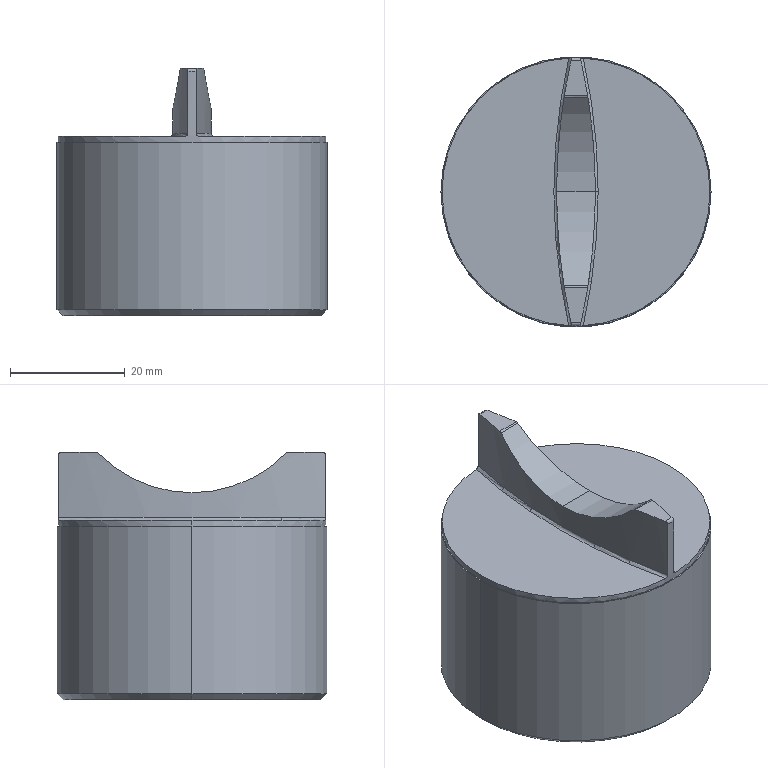Part | SolidWorks | features Fillet 3, ICE 3, Chamfer 1, Extrusion 1, HoleWzd 1 | 1 solid | 28 faces | box 47 x 47 x 43 mm | volume 54544 mm3 | cylinder 13 | plane 6 | torus 5 | cone 4 | commonest cylinder face diameters 210.861 x3 1 x2 8.5 x2 45.893 x2 46.6 x2 47 x2
STEP:
#1=CARTESIAN_POINT('',(-22.5,0.,0.));
#2=VERTEX_POINT('',#1);
#3=CARTESIAN_POINT('',(22.5,0.,0.));
#4=VERTEX_POINT('',#3);
#5=CARTESIAN_POINT('',(0.,0.,0.));
#6=DIRECTION('',(0.,0.,-1.));
#7=DIRECTION('',(1.,0.,0.));
#8=AXIS2_PLACEMENT_3D('',#5,#6,#7);
#9=CIRCLE('',#8,22.5);
#10=EDGE_CURVE('',#2,#4,#9,.T.);
#11=ORIENTED_EDGE('',*,*,#10,.F.);
#12=CARTESIAN_POINT('',(-23.5,0.,1.));
#13=VERTEX_POINT('',#12);
#14=CARTESIAN_POINT('',(-23.5,0.,1.));
#15=DIRECTION('',(-0.7071,0.,0.7071));
#16=VECTOR('',#15,1000.);
#17=LINE('',#14,#16);
#18=EDGE_CURVE('',#2,#13,#17,.T.);
#19=ORIENTED_EDGE('',*,*,#18,.T.);
#20=CARTESIAN_POINT('',(23.5,0.,1.));
#21=VERTEX_POINT('',#20);
#22=CARTESIAN_POINT('',(0.,0.,1.));
#23=DIRECTION('',(0.,0.,1.));
#24=DIRECTION('',(1.,0.,0.));
#25=AXIS2_PLACEMENT_3D('',#22,#23,#24);
#26=CIRCLE('',#25,23.5);
#27=EDGE_CURVE('',#21,#13,#26,.T.);
#28=ORIENTED_EDGE('',*,*,#27,.F.);
#29=CARTESIAN_POINT('',(23.5,0.,1.));
#30=DIRECTION('',(0.7071,0.,0.7071));
#31=VECTOR('',#30,1000.);
#32=LINE('',#29,#31);
#33=EDGE_CURVE('',#4,#21,#32,.T.);
#34=ORIENTED_EDGE('',*,*,#33,.F.);
#35=EDGE_LOOP('',(#11,#19,#28,#34));
#36=FACE_OUTER_BOUND('',#35,.T.);
#37=CARTESIAN_POINT('',(0.,0.,1.));
#38=DIRECTION('',(0.,0.,1.));
#39=DIRECTION('',(1.,0.,0.));
#40=AXIS2_PLACEMENT_3D('',#37,#38,#39);
#41=CONICAL_SURFACE('',#40,23.5,0.7854);
#42=ADVANCED_FACE('',(#36),#41,.T.);
#43=CARTESIAN_POINT('',(0.7458,-23.288,31.7));
#44=VERTEX_POINT('',#43);
#45=CARTESIAN_POINT('',(3.35,0.,31.7));
#46=VERTEX_POINT('',#45);
#47=CARTESIAN_POINT('',(-102.081,0.,31.7));
#48=DIRECTION('',(0.,0.,1.));
#49=DIRECTION('',(1.,0.,0.));
#50=AXIS2_PLACEMENT_3D('',#47,#48,#49);
#51=CIRCLE('',#50,105.431);
#52=EDGE_CURVE('',#44,#46,#51,.T.);
#53=ORIENTED_EDGE('',*,*,#52,.T.);
#54=CARTESIAN_POINT('',(3.35,0.,36.));
#55=VERTEX_POINT('',#54);
#56=CARTESIAN_POINT('',(3.35,0.,31.2));
#57=DIRECTION('',(0.,0.,1.));
#58=VECTOR('',#57,1000.);
#59=LINE('',#56,#58);
#60=EDGE_CURVE('',#46,#55,#59,.T.);
#61=ORIENTED_EDGE('',*,*,#60,.T.);
#62=CARTESIAN_POINT('',(2.074,-16.354,42.851));
#63=VERTEX_POINT('',#62);
#64=CARTESIAN_POINT('',(2.074,-16.354,42.851));
#65=CARTESIAN_POINT('',(2.242,-15.285,41.764));
#66=CARTESIAN_POINT('',(2.407,-14.125,40.8));
#67=CARTESIAN_POINT('',(2.637,-12.253,39.531));
#68=CARTESIAN_POINT('',(2.711,-11.607,39.137));
#69=CARTESIAN_POINT('',(2.816,-10.603,38.593));
#70=CARTESIAN_POINT('',(2.85,-10.262,38.419));
#71=CARTESIAN_POINT('',(2.915,-9.574,38.089));
#72=CARTESIAN_POINT('',(2.946,-9.227,37.933));
#73=CARTESIAN_POINT('',(3.094,-7.478,37.2));
#74=CARTESIAN_POINT('',(3.188,-6.034,36.755));
#75=CARTESIAN_POINT('',(3.268,-4.172,36.379));
#76=CARTESIAN_POINT('',(3.282,-3.797,36.313));
#77=CARTESIAN_POINT('',(3.307,-3.04,36.199));
#78=CARTESIAN_POINT('',(3.317,-2.658,36.151));
#79=CARTESIAN_POINT('',(3.342,-1.517,36.037));
#80=CARTESIAN_POINT('',(3.35,-0.7577,36.));
#81=CARTESIAN_POINT('',(3.35,0.,36.));
#82=B_SPLINE_CURVE_WITH_KNOTS('',3,(#64,#65,#66,#67,#68,#69,#70,#71,#72,#73,#74,#75,#76,#77,#78,#79,#80,#81),.UNSPECIFIED.,.F.,.F.,(4,2,2,2,2,2,2,2,4),(0.000207,0.004751,0.007022,0.008158,0.009294,0.01384,0.01497,0.01611,0.01838),.UNSPECIFIED.);
#83=EDGE_CURVE('',#63,#55,#82,.T.);
#84=ORIENTED_EDGE('',*,*,#83,.F.);
#85=CARTESIAN_POINT('',(2.017,-16.711,43.));
#86=VERTEX_POINT('',#85);
#87=CARTESIAN_POINT('',(2.074,-16.354,42.851));
#88=CARTESIAN_POINT('',(2.059,-16.448,42.946));
#89=CARTESIAN_POINT('',(2.039,-16.578,43.));
#90=CARTESIAN_POINT('',(2.017,-16.711,43.));
#91=B_SPLINE_CURVE_WITH_KNOTS('',3,(#87,#88,#89,#90),.UNSPECIFIED.,.F.,.F.,(4,4),(0.,0.0003983),.UNSPECIFIED.);
#92=EDGE_CURVE('',#63,#86,#91,.T.);
#93=ORIENTED_EDGE('',*,*,#92,.T.);
#94=CARTESIAN_POINT('',(0.8587,-22.784,43.));
#95=VERTEX_POINT('',#94);
#96=CARTESIAN_POINT('',(-102.081,0.,43.));
#97=DIRECTION('',(0.,0.,1.));
#98=DIRECTION('',(1.,0.,0.));
#99=AXIS2_PLACEMENT_3D('',#96,#97,#98);
#100=CIRCLE('',#99,105.431);
#101=EDGE_CURVE('',#95,#86,#100,.T.);
#102=ORIENTED_EDGE('',*,*,#101,.F.);
#103=CARTESIAN_POINT('',(0.7458,-23.288,42.5));
#104=VERTEX_POINT('',#103);
#105=CARTESIAN_POINT('',(0.8587,-22.784,43.));
#106=CARTESIAN_POINT('',(0.8297,-22.915,43.));
#107=CARTESIAN_POINT('',(0.801,-23.043,42.948));
#108=CARTESIAN_POINT('',(0.7587,-23.231,42.765));
#109=CARTESIAN_POINT('',(0.7458,-23.288,42.634));
#110=CARTESIAN_POINT('',(0.7458,-23.288,42.5));
#111=B_SPLINE_CURVE_WITH_KNOTS('',3,(#105,#106,#107,#108,#109,#110),.UNSPECIFIED.,.F.,.F.,(4,2,4),(0.,0.0003971,0.0007942),.UNSPECIFIED.);
#112=EDGE_CURVE('',#95,#104,#111,.T.);
#113=ORIENTED_EDGE('',*,*,#112,.T.);
#114=CARTESIAN_POINT('',(0.7458,-23.288,96.2));
#115=DIRECTION('',(0.,0.,1.));
#116=VECTOR('',#115,1000.);
#117=LINE('',#114,#116);
#118=EDGE_CURVE('',#44,#104,#117,.T.);
#119=ORIENTED_EDGE('',*,*,#118,.F.);
#120=EDGE_LOOP('',(#53,#61,#84,#93,#102,#113,#119));
#121=FACE_OUTER_BOUND('',#120,.T.);
#122=CARTESIAN_POINT('',(-102.081,0.,31.2));
#123=DIRECTION('',(0.,0.,1.));
#124=DIRECTION('',(1.,0.,0.));
#125=AXIS2_PLACEMENT_3D('',#122,#123,#124);
#126=CYLINDRICAL_SURFACE('',#125,105.431);
#127=ADVANCED_FACE('',(#121),#126,.T.);
#128=CARTESIAN_POINT('',(-3.35,0.,36.));
#129=VERTEX_POINT('',#128);
#130=CARTESIAN_POINT('',(-2.074,16.354,42.851));
#131=VERTEX_POINT('',#130);
#132=CARTESIAN_POINT('',(-3.35,0.,36.));
#133=CARTESIAN_POINT('',(-3.35,1.514,36.));
#134=CARTESIAN_POINT('',(-3.317,3.022,36.148));
#135=CARTESIAN_POINT('',(-3.221,5.274,36.601));
#136=CARTESIAN_POINT('',(-3.181,6.014,36.789));
#137=CARTESIAN_POINT('',(-3.088,7.462,37.234));
#138=CARTESIAN_POINT('',(-3.035,8.172,37.491));
#139=CARTESIAN_POINT('',(-2.918,9.565,38.075));
#140=CARTESIAN_POINT('',(-2.853,10.247,38.401));
#141=CARTESIAN_POINT('',(-2.714,11.584,39.124));
#142=CARTESIAN_POINT('',(-2.639,12.239,39.521));
#143=CARTESIAN_POINT('',(-2.407,14.123,40.798));
#144=CARTESIAN_POINT('',(-2.242,15.286,41.765));
#145=CARTESIAN_POINT('',(-2.074,16.354,42.851));
#146=B_SPLINE_CURVE_WITH_KNOTS('',3,(#132,#133,#134,#135,#136,#137,#138,#139,#140,#141,#142,#143,#144,#145),.UNSPECIFIED.,.F.,.F.,(4,2,2,2,2,2,4),(0.01838,0.02292,0.02519,0.02746,0.02973,0.032,0.03654),.UNSPECIFIED.);
#147=EDGE_CURVE('',#129,#131,#146,.T.);
#148=ORIENTED_EDGE('',*,*,#147,.F.);
#149=CARTESIAN_POINT('',(-6.,0.,36.));
#150=DIRECTION('',(1.,0.,0.));
#151=VECTOR('',#150,1000.);
#152=LINE('',#149,#151);
#153=EDGE_CURVE('',#129,#55,#152,.T.);
#154=ORIENTED_EDGE('',*,*,#153,.T.);
#155=CARTESIAN_POINT('',(2.074,16.354,42.851));
#156=VERTEX_POINT('',#155);
#157=CARTESIAN_POINT('',(3.35,0.,36.));
#158=CARTESIAN_POINT('',(3.35,1.514,36.));
#159=CARTESIAN_POINT('',(3.317,3.022,36.148));
#160=CARTESIAN_POINT('',(3.221,5.274,36.601));
#161=CARTESIAN_POINT('',(3.181,6.014,36.789));
#162=CARTESIAN_POINT('',(3.088,7.462,37.234));
#163=CARTESIAN_POINT('',(3.035,8.172,37.491));
#164=CARTESIAN_POINT('',(2.918,9.565,38.075));
#165=CARTESIAN_POINT('',(2.853,10.247,38.401));
#166=CARTESIAN_POINT('',(2.714,11.584,39.124));
#167=CARTESIAN_POINT('',(2.639,12.239,39.521));
#168=CARTESIAN_POINT('',(2.407,14.123,40.798));
#169=CARTESIAN_POINT('',(2.242,15.286,41.765));
#170=CARTESIAN_POINT('',(2.074,16.354,42.851));
#171=B_SPLINE_CURVE_WITH_KNOTS('',3,(#157,#158,#159,#160,#161,#162,#163,#164,#165,#166,#167,#168,#169,#170),.UNSPECIFIED.,.F.,.F.,(4,2,2,2,2,2,4),(0.01838,0.02292,0.02519,0.02746,0.02973,0.032,0.03654),.UNSPECIFIED.);
#172=EDGE_CURVE('',#55,#156,#171,.T.);
#173=ORIENTED_EDGE('',*,*,#172,.T.);
#174=CARTESIAN_POINT('',(-6.,16.354,42.851));
#175=DIRECTION('',(-1.,0.,0.));
#176=VECTOR('',#175,1000.);
#177=LINE('',#174,#176);
#178=EDGE_CURVE('',#156,#131,#177,.T.);
#179=ORIENTED_EDGE('',*,*,#178,.T.);
#180=EDGE_LOOP('',(#148,#154,#173,#179));
#181=FACE_OUTER_BOUND('',#180,.T.);
#182=CARTESIAN_POINT('',(-6.,0.,58.946));
#183=DIRECTION('',(1.,0.,0.));
#184=DIRECTION('',(0.,0.,-1.));
#185=AXIS2_PLACEMENT_3D('',#182,#183,#184);
#186=CYLINDRICAL_SURFACE('',#185,22.946);
#187=ADVANCED_FACE('',(#181),#186,.F.);
#188=CARTESIAN_POINT('',(1.263,23.266,31.2));
#189=VERTEX_POINT('',#188);
#190=CARTESIAN_POINT('',(23.3,0.,31.2));
#191=VERTEX_POINT('',#190);
#192=CARTESIAN_POINT('',(0.,0.,31.2));
#193=DIRECTION('',(0.,0.,-1.));
#194=DIRECTION('',(1.,0.,0.));
#195=AXIS2_PLACEMENT_3D('',#192,#193,#194);
#196=CIRCLE('',#195,23.3);
#197=EDGE_CURVE('',#189,#191,#196,.T.);
#198=ORIENTED_EDGE('',*,*,#197,.T.);
#199=CARTESIAN_POINT('',(23.3,0.,30.2));
#200=VERTEX_POINT('',#199);
#201=CARTESIAN_POINT('',(23.3,0.,162.2));
#202=DIRECTION('',(0.,0.,-1.));
#203=VECTOR('',#202,1000.);
#204=LINE('',#201,#203);
#205=EDGE_CURVE('',#191,#200,#204,.T.);
#206=ORIENTED_EDGE('',*,*,#205,.T.);
#207=CARTESIAN_POINT('',(-23.3,0.,30.2));
#208=VERTEX_POINT('',#207);
#209=CARTESIAN_POINT('',(0.,0.,30.2));
#210=DIRECTION('',(0.,0.,1.));
#211=DIRECTION('',(1.,0.,0.));
#212=AXIS2_PLACEMENT_3D('',#209,#210,#211);
#213=CIRCLE('',#212,23.3);
#214=EDGE_CURVE('',#200,#208,#213,.T.);
#215=ORIENTED_EDGE('',*,*,#214,.T.);
#216=CARTESIAN_POINT('',(-23.3,0.,31.2));
#217=VERTEX_POINT('',#216);
#218=CARTESIAN_POINT('',(-23.3,0.,162.2));
#219=DIRECTION('',(0.,0.,-1.));
#220=VECTOR('',#219,1000.);
#221=LINE('',#218,#220);
#222=EDGE_CURVE('',#217,#208,#221,.T.);
#223=ORIENTED_EDGE('',*,*,#222,.F.);
#224=CARTESIAN_POINT('',(-1.263,23.266,31.2));
#225=VERTEX_POINT('',#224);
#226=CARTESIAN_POINT('',(0.,0.,31.2));
#227=DIRECTION('',(0.,0.,-1.));
#228=DIRECTION('',(1.,0.,0.));
#229=AXIS2_PLACEMENT_3D('',#226,#227,#228);
#230=CIRCLE('',#229,23.3);
#231=EDGE_CURVE('',#217,#225,#230,.T.);
#232=ORIENTED_EDGE('',*,*,#231,.T.);
#233=CARTESIAN_POINT('',(-0.7458,23.288,31.7));
#234=VERTEX_POINT('',#233);
#235=CARTESIAN_POINT('',(-0.7458,23.288,31.7));
#236=CARTESIAN_POINT('',(-0.7458,23.288,31.567));
#237=CARTESIAN_POINT('',(-0.804,23.286,31.435));
#238=CARTESIAN_POINT('',(-0.9971,23.279,31.252));
#239=CARTESIAN_POINT('',(-1.129,23.273,31.2));
#240=CARTESIAN_POINT('',(-1.263,23.266,31.2));
#241=B_SPLINE_CURVE_WITH_KNOTS('',3,(#235,#236,#237,#238,#239,#240),.UNSPECIFIED.,.F.,.F.,(4,2,4),(0.00007147,0.0004697,0.000868),.UNSPECIFIED.);
#242=EDGE_CURVE('',#234,#225,#241,.T.);
#243=ORIENTED_EDGE('',*,*,#242,.F.);
#244=CARTESIAN_POINT('',(-0.7458,23.288,42.5));
#245=VERTEX_POINT('',#244);
#246=CARTESIAN_POINT('',(-0.7458,23.288,96.2));
#247=DIRECTION('',(0.,0.,-1.));
#248=VECTOR('',#247,1000.);
#249=LINE('',#246,#248);
#250=EDGE_CURVE('',#245,#234,#249,.T.);
#251=ORIENTED_EDGE('',*,*,#250,.F.);
#252=CARTESIAN_POINT('',(0.7458,23.288,42.5));
#253=VERTEX_POINT('',#252);
#254=CARTESIAN_POINT('',(0.,0.,42.5));
#255=DIRECTION('',(0.,0.,-1.));
#256=DIRECTION('',(1.,0.,0.));
#257=AXIS2_PLACEMENT_3D('',#254,#255,#256);
#258=CIRCLE('',#257,23.3);
#259=EDGE_CURVE('',#245,#253,#258,.T.);
#260=ORIENTED_EDGE('',*,*,#259,.T.);
#261=CARTESIAN_POINT('',(0.7458,23.288,31.7));
#262=VERTEX_POINT('',#261);
#263=CARTESIAN_POINT('',(0.7458,23.288,96.2));
#264=DIRECTION('',(0.,0.,-1.));
#265=VECTOR('',#264,1000.);
#266=LINE('',#263,#265);
#267=EDGE_CURVE('',#253,#262,#266,.T.);
#268=ORIENTED_EDGE('',*,*,#267,.T.);
#269=CARTESIAN_POINT('',(1.263,23.266,31.2));
#270=CARTESIAN_POINT('',(1.131,23.273,31.2));
#271=CARTESIAN_POINT('',(0.9971,23.279,31.252));
#272=CARTESIAN_POINT('',(0.8044,23.286,31.434));
#273=CARTESIAN_POINT('',(0.7458,23.288,31.565));
#274=CARTESIAN_POINT('',(0.7458,23.288,31.7));
#275=B_SPLINE_CURVE_WITH_KNOTS('',3,(#269,#270,#271,#272,#273,#274),.UNSPECIFIED.,.F.,.F.,(4,2,4),(0.00004476,0.0004428,0.0008408),.UNSPECIFIED.);
#276=EDGE_CURVE('',#189,#262,#275,.T.);
#277=ORIENTED_EDGE('',*,*,#276,.F.);
#278=EDGE_LOOP('',(#198,#206,#215,#223,#232,#243,#251,#260,#268,#277));
#279=FACE_OUTER_BOUND('',#278,.T.);
#280=CARTESIAN_POINT('',(0.,0.,162.2));
#281=DIRECTION('',(0.,0.,-1.));
#282=DIRECTION('',(-1.,0.,0.));
#283=AXIS2_PLACEMENT_3D('',#280,#281,#282);
#284=CYLINDRICAL_SURFACE('',#283,23.3);
#285=ADVANCED_FACE('',(#279),#284,.T.);
#286=CARTESIAN_POINT('',(4.25,0.,21.));
#287=VERTEX_POINT('',#286);
#288=CARTESIAN_POINT('',(-4.25,0.,21.));
#289=VERTEX_POINT('',#288);
#290=CARTESIAN_POINT('',(0.,0.,21.));
#291=DIRECTION('',(0.,0.,-1.));
#292=DIRECTION('',(-1.,0.,0.));
#293=AXIS2_PLACEMENT_3D('',#290,#291,#292);
#294=CIRCLE('',#293,4.25);
#295=EDGE_CURVE('',#287,#289,#294,.T.);
#296=ORIENTED_EDGE('',*,*,#295,.F.);
#297=CARTESIAN_POINT('',(4.25,0.,0.));
#298=VERTEX_POINT('',#297);
#299=CARTESIAN_POINT('',(4.25,0.,0.));
#300=DIRECTION('',(0.,0.,-1.));
#301=VECTOR('',#300,1000.);
#302=LINE('',#299,#301);
#303=EDGE_CURVE('',#287,#298,#302,.T.);
#304=ORIENTED_EDGE('',*,*,#303,.T.);
#305=CARTESIAN_POINT('',(-4.25,0.,0.));
#306=VERTEX_POINT('',#305);
#307=CARTESIAN_POINT('',(0.,0.,0.));
#308=DIRECTION('',(0.,0.,-1.));
#309=DIRECTION('',(-1.,0.,0.));
#310=AXIS2_PLACEMENT_3D('',#307,#308,#309);
#311=CIRCLE('',#310,4.25);
#312=EDGE_CURVE('',#298,#306,#311,.T.);
#313=ORIENTED_EDGE('',*,*,#312,.T.);
#314=CARTESIAN_POINT('',(-4.25,0.,0.));
#315=DIRECTION('',(0.,0.,-1.));
#316=VECTOR('',#315,1000.);
#317=LINE('',#314,#316);
#318=EDGE_CURVE('',#289,#306,#317,.T.);
#319=ORIENTED_EDGE('',*,*,#318,.F.);
#320=EDGE_LOOP('',(#296,#304,#313,#319));
#321=FACE_OUTER_BOUND('',#320,.T.);
#322=CARTESIAN_POINT('',(0.,0.,0.));
#323=DIRECTION('',(0.,0.,-1.));
#324=DIRECTION('',(-1.,0.,0.));
#325=AXIS2_PLACEMENT_3D('',#322,#323,#324);
#326=CYLINDRICAL_SURFACE('',#325,4.25);
#327=ADVANCED_FACE('',(#321),#326,.F.);
#328=CARTESIAN_POINT('',(0.,0.,23.554));
#329=VERTEX_POINT('',#328);
#330=CARTESIAN_POINT('',(-4.25,0.,21.));
#331=DIRECTION('',(-0.8572,0.,-0.515));
#332=VECTOR('',#331,1000.);
#333=LINE('',#330,#332);
#334=EDGE_CURVE('',#329,#289,#333,.T.);
#335=ORIENTED_EDGE('',*,*,#334,.F.);
#336=CARTESIAN_POINT('',(4.25,0.,21.));
#337=DIRECTION('',(0.8572,0.,-0.515));
#338=VECTOR('',#337,1000.);
#339=LINE('',#336,#338);
#340=EDGE_CURVE('',#329,#287,#339,.T.);
#341=ORIENTED_EDGE('',*,*,#340,.T.);
#342=ORIENTED_EDGE('',*,*,#295,.T.);
#343=EDGE_LOOP('',(#335,#341,#342));
#344=FACE_OUTER_BOUND('',#343,.T.);
#345=CARTESIAN_POINT('',(0.,0.,21.));
#346=DIRECTION('',(0.,0.,-1.));
#347=DIRECTION('',(-1.,0.,0.));
#348=AXIS2_PLACEMENT_3D('',#345,#346,#347);
#349=CONICAL_SURFACE('',#348,4.25,1.03);
#350=ADVANCED_FACE('',(#344),#349,.F.);
#351=CARTESIAN_POINT('',(23.5,0.,30.2));
#352=VERTEX_POINT('',#351);
#353=CARTESIAN_POINT('',(-23.5,0.,30.2));
#354=VERTEX_POINT('',#353);
#355=CARTESIAN_POINT('',(0.,0.,30.2));
#356=DIRECTION('',(0.,0.,1.));
#357=DIRECTION('',(1.,0.,0.));
#358=AXIS2_PLACEMENT_3D('',#355,#356,#357);
#359=CIRCLE('',#358,23.5);
#360=EDGE_CURVE('',#352,#354,#359,.T.);
#361=ORIENTED_EDGE('',*,*,#360,.F.);
#362=CARTESIAN_POINT('',(23.5,0.,43.));
#363=DIRECTION('',(0.,0.,-1.));
#364=VECTOR('',#363,1000.);
#365=LINE('',#362,#364);
#366=EDGE_CURVE('',#352,#21,#365,.T.);
#367=ORIENTED_EDGE('',*,*,#366,.T.);
#368=ORIENTED_EDGE('',*,*,#27,.T.);
#369=CARTESIAN_POINT('',(-23.5,0.,43.));
#370=DIRECTION('',(0.,0.,-1.));
#371=VECTOR('',#370,1000.);
#372=LINE('',#369,#371);
#373=EDGE_CURVE('',#354,#13,#372,.T.);
#374=ORIENTED_EDGE('',*,*,#373,.F.);
#375=EDGE_LOOP('',(#361,#367,#368,#374));
#376=FACE_OUTER_BOUND('',#375,.T.);
#377=CARTESIAN_POINT('',(0.,0.,43.));
#378=DIRECTION('',(0.,0.,-1.));
#379=DIRECTION('',(-1.,0.,0.));
#380=AXIS2_PLACEMENT_3D('',#377,#378,#379);
#381=CYLINDRICAL_SURFACE('',#380,23.5);
#382=ADVANCED_FACE('',(#376),#381,.T.);
#383=CARTESIAN_POINT('',(-102.081,0.,31.7));
#384=DIRECTION('',(0.,0.,1.));
#385=DIRECTION('',(1.,0.,0.));
#386=AXIS2_PLACEMENT_3D('',#383,#384,#385);
#387=CIRCLE('',#386,105.431);
#388=EDGE_CURVE('',#46,#262,#387,.T.);
#389=ORIENTED_EDGE('',*,*,#388,.F.);
#390=CARTESIAN_POINT('',(3.85,0.,31.2));
#391=VERTEX_POINT('',#390);
#392=CARTESIAN_POINT('',(3.85,0.,31.7));
#393=DIRECTION('',(0.,-1.,0.));
#394=DIRECTION('',(0.,0.,-1.));
#395=AXIS2_PLACEMENT_3D('',#392,#393,#394);
#396=CIRCLE('',#395,0.5);
#397=EDGE_CURVE('',#46,#391,#396,.T.);
#398=ORIENTED_EDGE('',*,*,#397,.T.);
#399=CARTESIAN_POINT('',(-102.081,0.,31.2));
#400=DIRECTION('',(0.,0.,-1.));
#401=DIRECTION('',(1.,0.,0.));
#402=AXIS2_PLACEMENT_3D('',#399,#400,#401);
#403=CIRCLE('',#402,105.931);
#404=EDGE_CURVE('',#189,#391,#403,.T.);
#405=ORIENTED_EDGE('',*,*,#404,.F.);
#406=ORIENTED_EDGE('',*,*,#276,.T.);
#407=EDGE_LOOP('',(#389,#398,#405,#406));
#408=FACE_OUTER_BOUND('',#407,.T.);
#409=CARTESIAN_POINT('',(-102.081,0.,31.7));
#410=DIRECTION('',(0.,0.,1.));
#411=DIRECTION('',(1.,0.,0.));
#412=AXIS2_PLACEMENT_3D('',#409,#410,#411);
#413=TOROIDAL_SURFACE('',#412,105.931,0.5);
#414=ADVANCED_FACE('',(#408),#413,.F.);
#415=CARTESIAN_POINT('',(-0.7458,-23.288,31.7));
#416=VERTEX_POINT('',#415);
#417=CARTESIAN_POINT('',(102.081,0.,31.7));
#418=DIRECTION('',(0.,0.,1.));
#419=DIRECTION('',(1.,0.,0.));
#420=AXIS2_PLACEMENT_3D('',#417,#418,#419);
#421=CIRCLE('',#420,105.431);
#422=EDGE_CURVE('',#234,#416,#421,.T.);
#423=ORIENTED_EDGE('',*,*,#422,.F.);
#424=ORIENTED_EDGE('',*,*,#242,.T.);
#425=CARTESIAN_POINT('',(-1.263,-23.266,31.2));
#426=VERTEX_POINT('',#425);
#427=CARTESIAN_POINT('',(102.081,0.,31.2));
#428=DIRECTION('',(0.,0.,-1.));
#429=DIRECTION('',(1.,0.,0.));
#430=AXIS2_PLACEMENT_3D('',#427,#428,#429);
#431=CIRCLE('',#430,105.931);
#432=EDGE_CURVE('',#426,#225,#431,.T.);
#433=ORIENTED_EDGE('',*,*,#432,.F.);
#434=CARTESIAN_POINT('',(-1.263,-23.266,31.2));
#435=CARTESIAN_POINT('',(-1.131,-23.273,31.2));
#436=CARTESIAN_POINT('',(-0.9971,-23.279,31.252));
#437=CARTESIAN_POINT('',(-0.8044,-23.286,31.434));
#438=CARTESIAN_POINT('',(-0.7458,-23.288,31.565));
#439=CARTESIAN_POINT('',(-0.7458,-23.288,31.7));
#440=B_SPLINE_CURVE_WITH_KNOTS('',3,(#434,#435,#436,#437,#438,#439),.UNSPECIFIED.,.F.,.F.,(4,2,4),(0.00004476,0.0004428,0.0008408),.UNSPECIFIED.);
#441=EDGE_CURVE('',#426,#416,#440,.T.);
#442=ORIENTED_EDGE('',*,*,#441,.T.);
#443=EDGE_LOOP('',(#423,#424,#433,#442));
#444=FACE_OUTER_BOUND('',#443,.T.);
#445=CARTESIAN_POINT('',(102.081,0.,31.7));
#446=DIRECTION('',(0.,0.,1.));
#447=DIRECTION('',(1.,0.,0.));
#448=AXIS2_PLACEMENT_3D('',#445,#446,#447);
#449=TOROIDAL_SURFACE('',#448,105.931,0.5);
#450=ADVANCED_FACE('',(#444),#449,.F.);
#451=ORIENTED_EDGE('',*,*,#397,.F.);
#452=ORIENTED_EDGE('',*,*,#52,.F.);
#453=CARTESIAN_POINT('',(1.263,-23.266,31.2));
#454=VERTEX_POINT('',#453);
#455=CARTESIAN_POINT('',(0.7458,-23.288,31.7));
#456=CARTESIAN_POINT('',(0.7458,-23.288,31.567));
#457=CARTESIAN_POINT('',(0.804,-23.286,31.435));
#458=CARTESIAN_POINT('',(0.9971,-23.279,31.252));
#459=CARTESIAN_POINT('',(1.129,-23.273,31.2));
#460=CARTESIAN_POINT('',(1.263,-23.266,31.2));
#461=B_SPLINE_CURVE_WITH_KNOTS('',3,(#455,#456,#457,#458,#459,#460),.UNSPECIFIED.,.F.,.F.,(4,2,4),(0.00007147,0.0004697,0.000868),.UNSPECIFIED.);
#462=EDGE_CURVE('',#44,#454,#461,.T.);
#463=ORIENTED_EDGE('',*,*,#462,.T.);
#464=CARTESIAN_POINT('',(-102.081,0.,31.2));
#465=DIRECTION('',(0.,0.,-1.));
#466=DIRECTION('',(1.,0.,0.));
#467=AXIS2_PLACEMENT_3D('',#464,#465,#466);
#468=CIRCLE('',#467,105.931);
#469=EDGE_CURVE('',#391,#454,#468,.T.);
#470=ORIENTED_EDGE('',*,*,#469,.F.);
#471=EDGE_LOOP('',(#451,#452,#463,#470));
#472=FACE_OUTER_BOUND('',#471,.T.);
#473=CARTESIAN_POINT('',(-102.081,0.,31.7));
#474=DIRECTION('',(0.,0.,1.));
#475=DIRECTION('',(1.,0.,0.));
#476=AXIS2_PLACEMENT_3D('',#473,#474,#475);
#477=TOROIDAL_SURFACE('',#476,105.931,0.5);
#478=ADVANCED_FACE('',(#472),#477,.F.);
#479=ORIENTED_EDGE('',*,*,#366,.F.);
#480=CARTESIAN_POINT('',(0.,0.,30.2));
#481=DIRECTION('',(0.,0.,1.));
#482=DIRECTION('',(1.,0.,0.));
#483=AXIS2_PLACEMENT_3D('',#480,#481,#482);
#484=CIRCLE('',#483,23.5);
#485=EDGE_CURVE('',#354,#352,#484,.T.);
#486=ORIENTED_EDGE('',*,*,#485,.F.);
#487=ORIENTED_EDGE('',*,*,#373,.T.);
#488=CARTESIAN_POINT('',(0.,0.,1.));
#489=DIRECTION('',(0.,0.,1.));
#490=DIRECTION('',(1.,0.,0.));
#491=AXIS2_PLACEMENT_3D('',#488,#489,#490);
#492=CIRCLE('',#491,23.5);
#493=EDGE_CURVE('',#13,#21,#492,.T.);
#494=ORIENTED_EDGE('',*,*,#493,.T.);
#495=EDGE_LOOP('',(#479,#486,#487,#494));
#496=FACE_OUTER_BOUND('',#495,.T.);
#497=CARTESIAN_POINT('',(0.,0.,43.));
#498=DIRECTION('',(0.,0.,-1.));
#499=DIRECTION('',(-1.,0.,0.));
#500=AXIS2_PLACEMENT_3D('',#497,#498,#499);
#501=CYLINDRICAL_SURFACE('',#500,23.5);
#502=ADVANCED_FACE('',(#496),#501,.T.);
#503=CARTESIAN_POINT('',(0.,0.,0.));
#504=DIRECTION('',(0.,0.,-1.));
#505=DIRECTION('',(1.,0.,0.));
#506=AXIS2_PLACEMENT_3D('',#503,#504,#505);
#507=CIRCLE('',#506,22.5);
#508=EDGE_CURVE('',#4,#2,#507,.T.);
#509=ORIENTED_EDGE('',*,*,#508,.T.);
#510=ORIENTED_EDGE('',*,*,#10,.T.);
#511=EDGE_LOOP('',(#509,#510));
#512=FACE_OUTER_BOUND('',#511,.T.);
#513=CARTESIAN_POINT('',(0.,0.,0.));
#514=DIRECTION('',(0.,0.,-1.));
#515=DIRECTION('',(-1.,0.,0.));
#516=AXIS2_PLACEMENT_3D('',#513,#514,#515);
#517=CIRCLE('',#516,4.25);
#518=EDGE_CURVE('',#306,#298,#517,.T.);
#519=ORIENTED_EDGE('',*,*,#518,.F.);
#520=ORIENTED_EDGE('',*,*,#312,.F.);
#521=EDGE_LOOP('',(#519,#520));
#522=FACE_BOUND('',#521,.T.);
#523=CARTESIAN_POINT('',(0.,0.,0.));
#524=DIRECTION('',(0.,0.,1.));
#525=DIRECTION('',(1.,0.,0.));
#526=AXIS2_PLACEMENT_3D('',#523,#524,#525);
#527=PLANE('',#526);
#528=ADVANCED_FACE('',(#512,#522),#527,.F.);
#529=ORIENTED_EDGE('',*,*,#340,.F.);
#530=ORIENTED_EDGE('',*,*,#334,.T.);
#531=CARTESIAN_POINT('',(0.,0.,21.));
#532=DIRECTION('',(0.,0.,-1.));
#533=DIRECTION('',(-1.,0.,0.));
#534=AXIS2_PLACEMENT_3D('',#531,#532,#533);
#535=CIRCLE('',#534,4.25);
#536=EDGE_CURVE('',#289,#287,#535,.T.);
#537=ORIENTED_EDGE('',*,*,#536,.T.);
#538=EDGE_LOOP('',(#529,#530,#537));
#539=FACE_OUTER_BOUND('',#538,.T.);
#540=CARTESIAN_POINT('',(0.,0.,21.));
#541=DIRECTION('',(0.,0.,-1.));
#542=DIRECTION('',(-1.,0.,0.));
#543=AXIS2_PLACEMENT_3D('',#540,#541,#542);
#544=CONICAL_SURFACE('',#543,4.25,1.03);
#545=ADVANCED_FACE('',(#539),#544,.F.);
#546=ORIENTED_EDGE('',*,*,#303,.F.);
#547=ORIENTED_EDGE('',*,*,#536,.F.);
#548=ORIENTED_EDGE('',*,*,#318,.T.);
#549=ORIENTED_EDGE('',*,*,#518,.T.);
#550=EDGE_LOOP('',(#546,#547,#548,#549));
#551=FACE_OUTER_BOUND('',#550,.T.);
#552=CARTESIAN_POINT('',(0.,0.,0.));
#553=DIRECTION('',(0.,0.,-1.));
#554=DIRECTION('',(-1.,0.,0.));
#555=AXIS2_PLACEMENT_3D('',#552,#553,#554);
#556=CYLINDRICAL_SURFACE('',#555,4.25);
#557=ADVANCED_FACE('',(#551),#556,.F.);
#558=ORIENTED_EDGE('',*,*,#205,.F.);
#559=CARTESIAN_POINT('',(0.,0.,31.2));
#560=DIRECTION('',(0.,0.,-1.));
#561=DIRECTION('',(1.,0.,0.));
#562=AXIS2_PLACEMENT_3D('',#559,#560,#561);
#563=CIRCLE('',#562,23.3);
#564=EDGE_CURVE('',#191,#454,#563,.T.);
#565=ORIENTED_EDGE('',*,*,#564,.T.);
#566=ORIENTED_EDGE('',*,*,#462,.F.);
#567=ORIENTED_EDGE('',*,*,#118,.T.);
#568=CARTESIAN_POINT('',(-0.7458,-23.288,42.5));
#569=VERTEX_POINT('',#568);
#570=CARTESIAN_POINT('',(0.,0.,42.5));
#571=DIRECTION('',(0.,0.,-1.));
#572=DIRECTION('',(1.,0.,0.));
#573=AXIS2_PLACEMENT_3D('',#570,#571,#572);
#574=CIRCLE('',#573,23.3);
#575=EDGE_CURVE('',#104,#569,#574,.T.);
#576=ORIENTED_EDGE('',*,*,#575,.T.);
#577=CARTESIAN_POINT('',(-0.7458,-23.288,96.2));
#578=DIRECTION('',(0.,0.,1.));
#579=VECTOR('',#578,1000.);
#580=LINE('',#577,#579);
#581=EDGE_CURVE('',#416,#569,#580,.T.);
#582=ORIENTED_EDGE('',*,*,#581,.F.);
#583=ORIENTED_EDGE('',*,*,#441,.F.);
#584=CARTESIAN_POINT('',(0.,0.,31.2));
#585=DIRECTION('',(0.,0.,-1.));
#586=DIRECTION('',(1.,0.,0.));
#587=AXIS2_PLACEMENT_3D('',#584,#585,#586);
#588=CIRCLE('',#587,23.3);
#589=EDGE_CURVE('',#426,#217,#588,.T.);
#590=ORIENTED_EDGE('',*,*,#589,.T.);
#591=ORIENTED_EDGE('',*,*,#222,.T.);
#592=CARTESIAN_POINT('',(0.,0.,30.2));
#593=DIRECTION('',(0.,0.,1.));
#594=DIRECTION('',(1.,0.,0.));
#595=AXIS2_PLACEMENT_3D('',#592,#593,#594);
#596=CIRCLE('',#595,23.3);
#597=EDGE_CURVE('',#208,#200,#596,.T.);
#598=ORIENTED_EDGE('',*,*,#597,.T.);
#599=EDGE_LOOP('',(#558,#565,#566,#567,#576,#582,#583,#590,#591,#598));
#600=FACE_OUTER_BOUND('',#599,.T.);
#601=CARTESIAN_POINT('',(0.,0.,162.2));
#602=DIRECTION('',(0.,0.,-1.));
#603=DIRECTION('',(-1.,0.,0.));
#604=AXIS2_PLACEMENT_3D('',#601,#602,#603);
#605=CYLINDRICAL_SURFACE('',#604,23.3);
#606=ADVANCED_FACE('',(#600),#605,.T.);
#607=ORIENTED_EDGE('',*,*,#597,.F.);
#608=ORIENTED_EDGE('',*,*,#214,.F.);
#609=EDGE_LOOP('',(#607,#608));
#610=FACE_BOUND('',#609,.T.);
#611=ORIENTED_EDGE('',*,*,#485,.T.);
#612=ORIENTED_EDGE('',*,*,#360,.T.);
#613=EDGE_LOOP('',(#611,#612));
#614=FACE_OUTER_BOUND('',#613,.T.);
#615=CARTESIAN_POINT('',(0.,0.,30.2));
#616=DIRECTION('',(0.,0.,1.));
#617=DIRECTION('',(1.,0.,0.));
#618=AXIS2_PLACEMENT_3D('',#615,#616,#617);
#619=PLANE('',#618);
#620=ADVANCED_FACE('',(#610,#614),#619,.T.);
#621=ORIENTED_EDGE('',*,*,#153,.F.);
#622=CARTESIAN_POINT('',(-2.074,-16.354,42.851));
#623=VERTEX_POINT('',#622);
#624=CARTESIAN_POINT('',(-2.074,-16.354,42.851));
#625=CARTESIAN_POINT('',(-2.242,-15.285,41.764));
#626=CARTESIAN_POINT('',(-2.407,-14.125,40.8));
#627=CARTESIAN_POINT('',(-2.637,-12.253,39.531));
#628=CARTESIAN_POINT('',(-2.711,-11.607,39.137));
#629=CARTESIAN_POINT('',(-2.816,-10.603,38.593));
#630=CARTESIAN_POINT('',(-2.85,-10.262,38.419));
#631=CARTESIAN_POINT('',(-2.915,-9.574,38.089));
#632=CARTESIAN_POINT('',(-2.946,-9.227,37.933));
#633=CARTESIAN_POINT('',(-3.094,-7.478,37.2));
#634=CARTESIAN_POINT('',(-3.188,-6.034,36.755));
#635=CARTESIAN_POINT('',(-3.268,-4.172,36.379));
#636=CARTESIAN_POINT('',(-3.282,-3.797,36.313));
#637=CARTESIAN_POINT('',(-3.307,-3.04,36.199));
#638=CARTESIAN_POINT('',(-3.317,-2.658,36.151));
#639=CARTESIAN_POINT('',(-3.342,-1.517,36.037));
#640=CARTESIAN_POINT('',(-3.35,-0.7577,36.));
#641=CARTESIAN_POINT('',(-3.35,0.,36.));
#642=B_SPLINE_CURVE_WITH_KNOTS('',3,(#624,#625,#626,#627,#628,#629,#630,#631,#632,#633,#634,#635,#636,#637,#638,#639,#640,#641),.UNSPECIFIED.,.F.,.F.,(4,2,2,2,2,2,2,2,4),(0.000207,0.004751,0.007022,0.008158,0.009294,0.01384,0.01497,0.01611,0.01838),.UNSPECIFIED.);
#643=EDGE_CURVE('',#623,#129,#642,.T.);
#644=ORIENTED_EDGE('',*,*,#643,.F.);
#645=CARTESIAN_POINT('',(-6.,-16.354,42.851));
#646=DIRECTION('',(1.,0.,0.));
#647=VECTOR('',#646,1000.);
#648=LINE('',#645,#647);
#649=EDGE_CURVE('',#623,#63,#648,.T.);
#650=ORIENTED_EDGE('',*,*,#649,.T.);
#651=ORIENTED_EDGE('',*,*,#83,.T.);
#652=EDGE_LOOP('',(#621,#644,#650,#651));
#653=FACE_OUTER_BOUND('',#652,.T.);
#654=CARTESIAN_POINT('',(-6.,0.,58.946));
#655=DIRECTION('',(1.,0.,0.));
#656=DIRECTION('',(0.,0.,-1.));
#657=AXIS2_PLACEMENT_3D('',#654,#655,#656);
#658=CYLINDRICAL_SURFACE('',#657,22.946);
#659=ADVANCED_FACE('',(#653),#658,.F.);
#660=ORIENTED_EDGE('',*,*,#197,.F.);
#661=ORIENTED_EDGE('',*,*,#404,.T.);
#662=ORIENTED_EDGE('',*,*,#469,.T.);
#663=ORIENTED_EDGE('',*,*,#564,.F.);
#664=EDGE_LOOP('',(#660,#661,#662,#663));
#665=FACE_OUTER_BOUND('',#664,.T.);
#666=CARTESIAN_POINT('',(0.,0.,31.2));
#667=DIRECTION('',(0.,0.,1.));
#668=DIRECTION('',(1.,0.,0.));
#669=AXIS2_PLACEMENT_3D('',#666,#667,#668);
#670=PLANE('',#669);
#671=ADVANCED_FACE('',(#665),#670,.T.);
#672=ORIENTED_EDGE('',*,*,#60,.F.);
#673=ORIENTED_EDGE('',*,*,#388,.T.);
#674=ORIENTED_EDGE('',*,*,#267,.F.);
#675=CARTESIAN_POINT('',(0.8587,22.784,43.));
#676=VERTEX_POINT('',#675);
#677=CARTESIAN_POINT('',(0.7458,23.288,42.5));
#678=CARTESIAN_POINT('',(0.7458,23.288,42.634));
#679=CARTESIAN_POINT('',(0.7588,23.231,42.765));
#680=CARTESIAN_POINT('',(0.8009,23.044,42.948));
#681=CARTESIAN_POINT('',(0.8297,22.915,43.));
#682=CARTESIAN_POINT('',(0.8587,22.784,43.));
#683=B_SPLINE_CURVE_WITH_KNOTS('',3,(#677,#678,#679,#680,#681,#682),.UNSPECIFIED.,.F.,.F.,(4,2,4),(0.,0.0003971,0.0007942),.UNSPECIFIED.);
#684=EDGE_CURVE('',#253,#676,#683,.T.);
#685=ORIENTED_EDGE('',*,*,#684,.T.);
#686=CARTESIAN_POINT('',(2.017,16.711,43.));
#687=VERTEX_POINT('',#686);
#688=CARTESIAN_POINT('',(-102.081,0.,43.));
#689=DIRECTION('',(0.,0.,1.));
#690=DIRECTION('',(1.,0.,0.));
#691=AXIS2_PLACEMENT_3D('',#688,#689,#690);
#692=CIRCLE('',#691,105.431);
#693=EDGE_CURVE('',#687,#676,#692,.T.);
#694=ORIENTED_EDGE('',*,*,#693,.F.);
#695=CARTESIAN_POINT('',(2.017,16.711,43.));
#696=CARTESIAN_POINT('',(2.039,16.578,43.));
#697=CARTESIAN_POINT('',(2.059,16.448,42.946));
#698=CARTESIAN_POINT('',(2.074,16.354,42.851));
#699=B_SPLINE_CURVE_WITH_KNOTS('',3,(#695,#696,#697,#698),.UNSPECIFIED.,.F.,.F.,(4,4),(0.,0.0003984),.UNSPECIFIED.);
#700=EDGE_CURVE('',#687,#156,#699,.T.);
#701=ORIENTED_EDGE('',*,*,#700,.T.);
#702=ORIENTED_EDGE('',*,*,#172,.F.);
#703=EDGE_LOOP('',(#672,#673,#674,#685,#694,#701,#702));
#704=FACE_OUTER_BOUND('',#703,.T.);
#705=CARTESIAN_POINT('',(-102.081,0.,31.2));
#706=DIRECTION('',(0.,0.,1.));
#707=DIRECTION('',(1.,0.,0.));
#708=AXIS2_PLACEMENT_3D('',#705,#706,#707);
#709=CYLINDRICAL_SURFACE('',#708,105.431);
#710=ADVANCED_FACE('',(#704),#709,.T.);
#711=ORIENTED_EDGE('',*,*,#589,.F.);
#712=ORIENTED_EDGE('',*,*,#432,.T.);
#713=ORIENTED_EDGE('',*,*,#231,.F.);
#714=EDGE_LOOP('',(#711,#712,#713));
#715=FACE_OUTER_BOUND('',#714,.T.);
#716=CARTESIAN_POINT('',(0.,0.,31.2));
#717=DIRECTION('',(0.,0.,1.));
#718=DIRECTION('',(1.,0.,0.));
#719=AXIS2_PLACEMENT_3D('',#716,#717,#718);
#720=PLANE('',#719);
#721=ADVANCED_FACE('',(#715),#720,.T.);
#722=ORIENTED_EDGE('',*,*,#250,.T.);
#723=ORIENTED_EDGE('',*,*,#422,.T.);
#724=ORIENTED_EDGE('',*,*,#581,.T.);
#725=CARTESIAN_POINT('',(-0.8587,-22.784,43.));
#726=VERTEX_POINT('',#725);
#727=CARTESIAN_POINT('',(-0.7458,-23.288,42.5));
#728=CARTESIAN_POINT('',(-0.7458,-23.288,42.634));
#729=CARTESIAN_POINT('',(-0.7588,-23.231,42.765));
#730=CARTESIAN_POINT('',(-0.8009,-23.044,42.948));
#731=CARTESIAN_POINT('',(-0.8297,-22.915,43.));
#732=CARTESIAN_POINT('',(-0.8587,-22.784,43.));
#733=B_SPLINE_CURVE_WITH_KNOTS('',3,(#727,#728,#729,#730,#731,#732),.UNSPECIFIED.,.F.,.F.,(4,2,4),(0.,0.0003971,0.0007942),.UNSPECIFIED.);
#734=EDGE_CURVE('',#569,#726,#733,.T.);
#735=ORIENTED_EDGE('',*,*,#734,.T.);
#736=CARTESIAN_POINT('',(-2.017,-16.711,43.));
#737=VERTEX_POINT('',#736);
#738=CARTESIAN_POINT('',(102.081,0.,43.));
#739=DIRECTION('',(0.,0.,-1.));
#740=DIRECTION('',(1.,0.,0.));
#741=AXIS2_PLACEMENT_3D('',#738,#739,#740);
#742=CIRCLE('',#741,105.431);
#743=EDGE_CURVE('',#726,#737,#742,.T.);
#744=ORIENTED_EDGE('',*,*,#743,.T.);
#745=CARTESIAN_POINT('',(-2.017,-16.711,43.));
#746=CARTESIAN_POINT('',(-2.039,-16.578,43.));
#747=CARTESIAN_POINT('',(-2.059,-16.448,42.946));
#748=CARTESIAN_POINT('',(-2.074,-16.354,42.851));
#749=B_SPLINE_CURVE_WITH_KNOTS('',3,(#745,#746,#747,#748),.UNSPECIFIED.,.F.,.F.,(4,4),(0.,0.0003984),.UNSPECIFIED.);
#750=EDGE_CURVE('',#737,#623,#749,.T.);
#751=ORIENTED_EDGE('',*,*,#750,.T.);
#752=ORIENTED_EDGE('',*,*,#643,.T.);
#753=ORIENTED_EDGE('',*,*,#147,.T.);
#754=CARTESIAN_POINT('',(-2.017,16.711,43.));
#755=VERTEX_POINT('',#754);
#756=CARTESIAN_POINT('',(-2.074,16.354,42.851));
#757=CARTESIAN_POINT('',(-2.059,16.448,42.946));
#758=CARTESIAN_POINT('',(-2.039,16.578,43.));
#759=CARTESIAN_POINT('',(-2.017,16.711,43.));
#760=B_SPLINE_CURVE_WITH_KNOTS('',3,(#756,#757,#758,#759),.UNSPECIFIED.,.F.,.F.,(4,4),(0.,0.0003983),.UNSPECIFIED.);
#761=EDGE_CURVE('',#131,#755,#760,.T.);
#762=ORIENTED_EDGE('',*,*,#761,.T.);
#763=CARTESIAN_POINT('',(-0.8587,22.784,43.));
#764=VERTEX_POINT('',#763);
#765=CARTESIAN_POINT('',(102.081,0.,43.));
#766=DIRECTION('',(0.,0.,-1.));
#767=DIRECTION('',(1.,0.,0.));
#768=AXIS2_PLACEMENT_3D('',#765,#766,#767);
#769=CIRCLE('',#768,105.431);
#770=EDGE_CURVE('',#755,#764,#769,.T.);
#771=ORIENTED_EDGE('',*,*,#770,.T.);
#772=CARTESIAN_POINT('',(-0.8587,22.784,43.));
#773=CARTESIAN_POINT('',(-0.8297,22.915,43.));
#774=CARTESIAN_POINT('',(-0.801,23.043,42.948));
#775=CARTESIAN_POINT('',(-0.7587,23.231,42.765));
#776=CARTESIAN_POINT('',(-0.7458,23.288,42.634));
#777=CARTESIAN_POINT('',(-0.7458,23.288,42.5));
#778=B_SPLINE_CURVE_WITH_KNOTS('',3,(#772,#773,#774,#775,#776,#777),.UNSPECIFIED.,.F.,.F.,(4,2,4),(0.,0.0003971,0.0007942),.UNSPECIFIED.);
#779=EDGE_CURVE('',#764,#245,#778,.T.);
#780=ORIENTED_EDGE('',*,*,#779,.T.);
#781=EDGE_LOOP('',(#722,#723,#724,#735,#744,#751,#752,#753,#762,#771,#780));
#782=FACE_OUTER_BOUND('',#781,.T.);
#783=CARTESIAN_POINT('',(102.081,0.,31.2));
#784=DIRECTION('',(0.,0.,1.));
#785=DIRECTION('',(1.,0.,0.));
#786=AXIS2_PLACEMENT_3D('',#783,#784,#785);
#787=CYLINDRICAL_SURFACE('',#786,105.431);
#788=ADVANCED_FACE('',(#782),#787,.T.);
#789=ORIENTED_EDGE('',*,*,#770,.F.);
#790=CARTESIAN_POINT('',(2.051,16.711,43.));
#791=DIRECTION('',(1.,0.,0.));
#792=VECTOR('',#791,1000.);
#793=LINE('',#790,#792);
#794=EDGE_CURVE('',#755,#687,#793,.T.);
#795=ORIENTED_EDGE('',*,*,#794,.T.);
#796=ORIENTED_EDGE('',*,*,#693,.T.);
#797=CARTESIAN_POINT('',(0.,0.,43.));
#798=DIRECTION('',(0.,0.,1.));
#799=DIRECTION('',(1.,0.,0.));
#800=AXIS2_PLACEMENT_3D('',#797,#798,#799);
#801=CIRCLE('',#800,22.8);
#802=EDGE_CURVE('',#676,#764,#801,.T.);
#803=ORIENTED_EDGE('',*,*,#802,.T.);
#804=EDGE_LOOP('',(#789,#795,#796,#803));
#805=FACE_OUTER_BOUND('',#804,.T.);
#806=CARTESIAN_POINT('',(0.,0.,43.));
#807=DIRECTION('',(0.,0.,1.));
#808=DIRECTION('',(1.,0.,0.));
#809=AXIS2_PLACEMENT_3D('',#806,#807,#808);
#810=PLANE('',#809);
#811=ADVANCED_FACE('',(#805),#810,.T.);
#812=ORIENTED_EDGE('',*,*,#743,.F.);
#813=CARTESIAN_POINT('',(0.,0.,43.));
#814=DIRECTION('',(0.,0.,1.));
#815=DIRECTION('',(1.,0.,0.));
#816=AXIS2_PLACEMENT_3D('',#813,#814,#815);
#817=CIRCLE('',#816,22.8);
#818=EDGE_CURVE('',#726,#95,#817,.T.);
#819=ORIENTED_EDGE('',*,*,#818,.T.);
#820=ORIENTED_EDGE('',*,*,#101,.T.);
#821=CARTESIAN_POINT('',(-2.051,-16.711,43.));
#822=DIRECTION('',(-1.,0.,0.));
#823=VECTOR('',#822,1000.);
#824=LINE('',#821,#823);
#825=EDGE_CURVE('',#86,#737,#824,.T.);
#826=ORIENTED_EDGE('',*,*,#825,.T.);
#827=EDGE_LOOP('',(#812,#819,#820,#826));
#828=FACE_OUTER_BOUND('',#827,.T.);
#829=CARTESIAN_POINT('',(0.,0.,43.));
#830=DIRECTION('',(0.,0.,1.));
#831=DIRECTION('',(1.,0.,0.));
#832=AXIS2_PLACEMENT_3D('',#829,#830,#831);
#833=PLANE('',#832);
#834=ADVANCED_FACE('',(#828),#833,.T.);
#835=ORIENTED_EDGE('',*,*,#112,.F.);
#836=ORIENTED_EDGE('',*,*,#818,.F.);
#837=ORIENTED_EDGE('',*,*,#734,.F.);
#838=ORIENTED_EDGE('',*,*,#575,.F.);
#839=EDGE_LOOP('',(#835,#836,#837,#838));
#840=FACE_OUTER_BOUND('',#839,.T.);
#841=CARTESIAN_POINT('',(0.,0.,42.5));
#842=DIRECTION('',(0.,0.,1.));
#843=DIRECTION('',(1.,0.,0.));
#844=AXIS2_PLACEMENT_3D('',#841,#842,#843);
#845=TOROIDAL_SURFACE('',#844,22.8,0.5);
#846=ADVANCED_FACE('',(#840),#845,.T.);
#847=ORIENTED_EDGE('',*,*,#750,.F.);
#848=ORIENTED_EDGE('',*,*,#825,.F.);
#849=ORIENTED_EDGE('',*,*,#92,.F.);
#850=ORIENTED_EDGE('',*,*,#649,.F.);
#851=EDGE_LOOP('',(#847,#848,#849,#850));
#852=FACE_OUTER_BOUND('',#851,.T.);
#853=CARTESIAN_POINT('',(-6.,-16.711,42.5));
#854=DIRECTION('',(1.,0.,0.));
#855=DIRECTION('',(0.,0.,-1.));
#856=AXIS2_PLACEMENT_3D('',#853,#854,#855);
#857=CYLINDRICAL_SURFACE('',#856,0.5);
#858=ADVANCED_FACE('',(#852),#857,.T.);
#859=ORIENTED_EDGE('',*,*,#761,.F.);
#860=ORIENTED_EDGE('',*,*,#178,.F.);
#861=ORIENTED_EDGE('',*,*,#700,.F.);
#862=ORIENTED_EDGE('',*,*,#794,.F.);
#863=EDGE_LOOP('',(#859,#860,#861,#862));
#864=FACE_OUTER_BOUND('',#863,.T.);
#865=CARTESIAN_POINT('',(-6.,16.711,42.5));
#866=DIRECTION('',(1.,0.,0.));
#867=DIRECTION('',(0.,0.,-1.));
#868=AXIS2_PLACEMENT_3D('',#865,#866,#867);
#869=CYLINDRICAL_SURFACE('',#868,0.5);
#870=ADVANCED_FACE('',(#864),#869,.T.);
#871=ORIENTED_EDGE('',*,*,#779,.F.);
#872=ORIENTED_EDGE('',*,*,#802,.F.);
#873=ORIENTED_EDGE('',*,*,#684,.F.);
#874=ORIENTED_EDGE('',*,*,#259,.F.);
#875=EDGE_LOOP('',(#871,#872,#873,#874));
#876=FACE_OUTER_BOUND('',#875,.T.);
#877=CARTESIAN_POINT('',(0.,0.,42.5));
#878=DIRECTION('',(0.,0.,1.));
#879=DIRECTION('',(1.,0.,0.));
#880=AXIS2_PLACEMENT_3D('',#877,#878,#879);
#881=TOROIDAL_SURFACE('',#880,22.8,0.5);
#882=ADVANCED_FACE('',(#876),#881,.T.);
#883=ORIENTED_EDGE('',*,*,#18,.F.);
#884=ORIENTED_EDGE('',*,*,#508,.F.);
#885=ORIENTED_EDGE('',*,*,#33,.T.);
#886=ORIENTED_EDGE('',*,*,#493,.F.);
#887=EDGE_LOOP('',(#883,#884,#885,#886));
#888=FACE_OUTER_BOUND('',#887,.T.);
#889=CARTESIAN_POINT('',(0.,0.,1.));
#890=DIRECTION('',(0.,0.,1.));
#891=DIRECTION('',(1.,0.,0.));
#892=AXIS2_PLACEMENT_3D('',#889,#890,#891);
#893=CONICAL_SURFACE('',#892,23.5,0.7854);
#894=ADVANCED_FACE('',(#888),#893,.T.);
#895=CLOSED_SHELL('',(#42,#127,#187,#285,#327,#350,#382,#414,#450,#478,#502,#528,#545,#557,#606,#620,#659,#671,#710,#721,#788,#811,#834,#846,#858,#870,#882,#894));
#896=MANIFOLD_SOLID_BREP('',#895);
#897=CARTESIAN_POINT('',(0.,0.,0.));
#898=DIRECTION('',(0.,0.,1.));
#899=DIRECTION('',(1.,0.,0.));
#900=AXIS2_PLACEMENT_3D('',#897,#898,#899);
#901=(LENGTH_UNIT()NAMED_UNIT(*)SI_UNIT(.MILLI.,.METRE.));
#902=UNCERTAINTY_MEASURE_WITH_UNIT(LENGTH_MEASURE(0.00001),#901,'','');
#903=(NAMED_UNIT(*)PLANE_ANGLE_UNIT()SI_UNIT($,.RADIAN.));
#904=(NAMED_UNIT(*)SI_UNIT($,.STERADIAN.)SOLID_ANGLE_UNIT());
#905=(GEOMETRIC_REPRESENTATION_CONTEXT(3)GLOBAL_UNCERTAINTY_ASSIGNED_CONTEXT((#902))GLOBAL_UNIT_ASSIGNED_CONTEXT((#901,#903,#904))REPRESENTATION_CONTEXT('',''));
#906=ADVANCED_BREP_SHAPE_REPRESENTATION('',(#896,#900),#905);